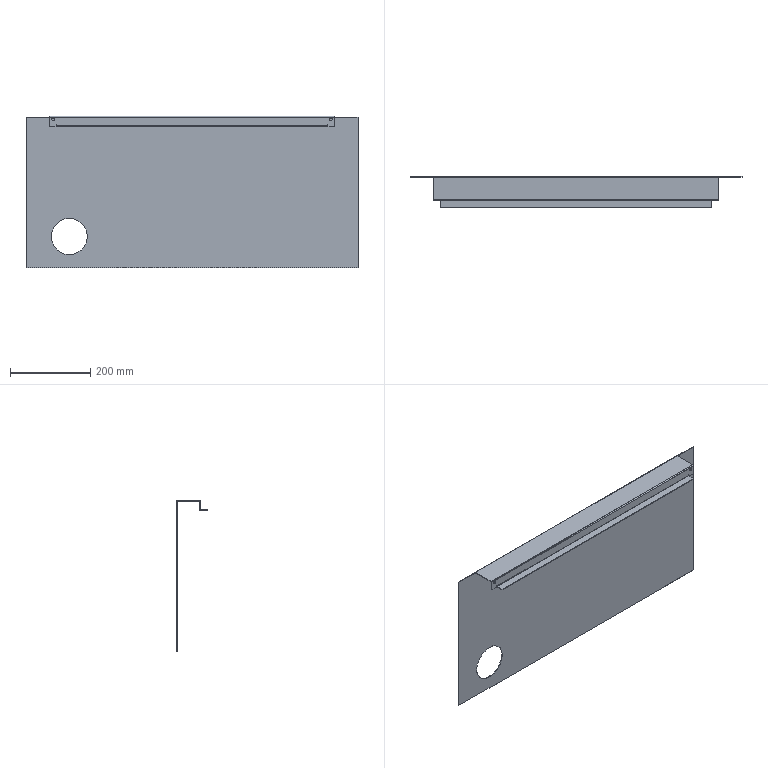Part | STEP file | Electrical Cabinet 3 | 1 solid | 42 faces | box 828 x 78 x 378 mm | volume 749579 mm3 | plane 24 | cylinder 18 | commonest cylinder face diameters 1 x9 7 x4 5 x3 90 x2
STEP:
#1=CARTESIAN_POINT('',(32.62,0.,79.307));
#2=VERTEX_POINT('',#1);
#3=CARTESIAN_POINT('',(32.62,0.,-10.693));
#4=VERTEX_POINT('',#3);
#5=CARTESIAN_POINT('',(32.62,0.,34.307));
#6=DIRECTION('',(0.,-1.,0.));
#7=DIRECTION('',(0.,0.,-1.));
#8=AXIS2_PLACEMENT_3D('',#5,#6,#7);
#9=CIRCLE('',#8,45.);
#10=EDGE_CURVE('',#2,#4,#9,.T.);
#11=ORIENTED_EDGE('',*,*,#10,.F.);
#12=CARTESIAN_POINT('',(32.62,-2.,79.307));
#13=VERTEX_POINT('',#12);
#14=CARTESIAN_POINT('',(32.62,8.,79.307));
#15=DIRECTION('',(0.,-1.,0.));
#16=VECTOR('',#15,1000.);
#17=LINE('',#14,#16);
#18=EDGE_CURVE('',#2,#13,#17,.T.);
#19=ORIENTED_EDGE('',*,*,#18,.T.);
#20=CARTESIAN_POINT('',(32.62,-2.,-10.693));
#21=VERTEX_POINT('',#20);
#22=CARTESIAN_POINT('',(32.62,-2.,34.307));
#23=DIRECTION('',(0.,-1.,0.));
#24=DIRECTION('',(0.,0.,-1.));
#25=AXIS2_PLACEMENT_3D('',#22,#23,#24);
#26=CIRCLE('',#25,45.);
#27=EDGE_CURVE('',#13,#21,#26,.T.);
#28=ORIENTED_EDGE('',*,*,#27,.T.);
#29=CARTESIAN_POINT('',(32.62,8.,-10.693));
#30=DIRECTION('',(0.,-1.,0.));
#31=VECTOR('',#30,1000.);
#32=LINE('',#29,#31);
#33=EDGE_CURVE('',#4,#21,#32,.T.);
#34=ORIENTED_EDGE('',*,*,#33,.F.);
#35=EDGE_LOOP('',(#11,#19,#28,#34));
#36=FACE_OUTER_BOUND('',#35,.T.);
#37=CARTESIAN_POINT('',(32.62,8.,34.307));
#38=DIRECTION('',(0.,-1.,0.));
#39=DIRECTION('',(0.,0.,-1.));
#40=AXIS2_PLACEMENT_3D('',#37,#38,#39);
#41=CYLINDRICAL_SURFACE('',#40,45.);
#42=ADVANCED_FACE('',(#36),#41,.F.);
#43=CARTESIAN_POINT('',(684.62,-58.,322.807));
#44=VERTEX_POINT('',#43);
#45=CARTESIAN_POINT('',(684.62,-58.,329.807));
#46=VERTEX_POINT('',#45);
#47=CARTESIAN_POINT('',(684.62,-58.,326.307));
#48=DIRECTION('',(0.,1.,0.));
#49=DIRECTION('',(0.,0.,-1.));
#50=AXIS2_PLACEMENT_3D('',#47,#48,#49);
#51=CIRCLE('',#50,3.5);
#52=EDGE_CURVE('',#44,#46,#51,.T.);
#53=ORIENTED_EDGE('',*,*,#52,.T.);
#54=CARTESIAN_POINT('',(684.62,-60.,329.807));
#55=VERTEX_POINT('',#54);
#56=CARTESIAN_POINT('',(684.62,-50.,329.807));
#57=DIRECTION('',(0.,-1.,0.));
#58=VECTOR('',#57,1000.);
#59=LINE('',#56,#58);
#60=EDGE_CURVE('',#46,#55,#59,.T.);
#61=ORIENTED_EDGE('',*,*,#60,.T.);
#62=CARTESIAN_POINT('',(684.62,-60.,322.807));
#63=VERTEX_POINT('',#62);
#64=CARTESIAN_POINT('',(684.62,-60.,326.307));
#65=DIRECTION('',(0.,1.,0.));
#66=DIRECTION('',(0.,0.,-1.));
#67=AXIS2_PLACEMENT_3D('',#64,#65,#66);
#68=CIRCLE('',#67,3.5);
#69=EDGE_CURVE('',#63,#55,#68,.T.);
#70=ORIENTED_EDGE('',*,*,#69,.F.);
#71=CARTESIAN_POINT('',(684.62,-50.,322.807));
#72=DIRECTION('',(0.,-1.,0.));
#73=VECTOR('',#72,1000.);
#74=LINE('',#71,#73);
#75=EDGE_CURVE('',#44,#63,#74,.T.);
#76=ORIENTED_EDGE('',*,*,#75,.F.);
#77=EDGE_LOOP('',(#53,#61,#70,#76));
#78=FACE_OUTER_BOUND('',#77,.T.);
#79=CARTESIAN_POINT('',(684.62,-50.,326.307));
#80=DIRECTION('',(0.,-1.,0.));
#81=DIRECTION('',(0.,0.,-1.));
#82=AXIS2_PLACEMENT_3D('',#79,#80,#81);
#83=CYLINDRICAL_SURFACE('',#82,3.5);
#84=ADVANCED_FACE('',(#78),#83,.F.);
#85=CARTESIAN_POINT('',(-7.38,-58.,322.807));
#86=VERTEX_POINT('',#85);
#87=CARTESIAN_POINT('',(-7.38,-58.,329.807));
#88=VERTEX_POINT('',#87);
#89=CARTESIAN_POINT('',(-7.38,-58.,326.307));
#90=DIRECTION('',(0.,1.,0.));
#91=DIRECTION('',(0.,0.,-1.));
#92=AXIS2_PLACEMENT_3D('',#89,#90,#91);
#93=CIRCLE('',#92,3.5);
#94=EDGE_CURVE('',#86,#88,#93,.T.);
#95=ORIENTED_EDGE('',*,*,#94,.T.);
#96=CARTESIAN_POINT('',(-7.38,-60.,329.807));
#97=VERTEX_POINT('',#96);
#98=CARTESIAN_POINT('',(-7.38,-50.,329.807));
#99=DIRECTION('',(0.,-1.,0.));
#100=VECTOR('',#99,1000.);
#101=LINE('',#98,#100);
#102=EDGE_CURVE('',#88,#97,#101,.T.);
#103=ORIENTED_EDGE('',*,*,#102,.T.);
#104=CARTESIAN_POINT('',(-7.38,-60.,322.807));
#105=VERTEX_POINT('',#104);
#106=CARTESIAN_POINT('',(-7.38,-60.,326.307));
#107=DIRECTION('',(0.,1.,0.));
#108=DIRECTION('',(0.,0.,-1.));
#109=AXIS2_PLACEMENT_3D('',#106,#107,#108);
#110=CIRCLE('',#109,3.5);
#111=EDGE_CURVE('',#105,#97,#110,.T.);
#112=ORIENTED_EDGE('',*,*,#111,.F.);
#113=CARTESIAN_POINT('',(-7.38,-50.,322.807));
#114=DIRECTION('',(0.,-1.,0.));
#115=VECTOR('',#114,1000.);
#116=LINE('',#113,#115);
#117=EDGE_CURVE('',#86,#105,#116,.T.);
#118=ORIENTED_EDGE('',*,*,#117,.F.);
#119=EDGE_LOOP('',(#95,#103,#112,#118));
#120=FACE_OUTER_BOUND('',#119,.T.);
#121=CARTESIAN_POINT('',(-7.38,-50.,326.307));
#122=DIRECTION('',(0.,-1.,0.));
#123=DIRECTION('',(0.,0.,-1.));
#124=AXIS2_PLACEMENT_3D('',#121,#122,#123);
#125=CYLINDRICAL_SURFACE('',#124,3.5);
#126=ADVANCED_FACE('',(#120),#125,.F.);
#127=CARTESIAN_POINT('',(677.12,-60.,313.307));
#128=VERTEX_POINT('',#127);
#129=CARTESIAN_POINT('',(677.62,-60.,312.807));
#130=VERTEX_POINT('',#129);
#131=CARTESIAN_POINT('',(677.12,-60.,312.807));
#132=DIRECTION('',(0.,1.,0.));
#133=DIRECTION('',(0.,0.,1.));
#134=AXIS2_PLACEMENT_3D('',#131,#132,#133);
#135=CIRCLE('',#134,0.5);
#136=EDGE_CURVE('',#128,#130,#135,.T.);
#137=ORIENTED_EDGE('',*,*,#136,.F.);
#138=CARTESIAN_POINT('',(677.12,-58.,313.307));
#139=VERTEX_POINT('',#138);
#140=CARTESIAN_POINT('',(677.12,-60.,313.307));
#141=DIRECTION('',(0.,1.,0.));
#142=VECTOR('',#141,1000.);
#143=LINE('',#140,#142);
#144=EDGE_CURVE('',#128,#139,#143,.T.);
#145=ORIENTED_EDGE('',*,*,#144,.T.);
#146=CARTESIAN_POINT('',(677.62,-58.,312.807));
#147=VERTEX_POINT('',#146);
#148=CARTESIAN_POINT('',(677.12,-58.,312.807));
#149=DIRECTION('',(0.,-1.,0.));
#150=DIRECTION('',(0.,0.,1.));
#151=AXIS2_PLACEMENT_3D('',#148,#149,#150);
#152=CIRCLE('',#151,0.5);
#153=EDGE_CURVE('',#147,#139,#152,.T.);
#154=ORIENTED_EDGE('',*,*,#153,.F.);
#155=CARTESIAN_POINT('',(677.62,-60.,312.807));
#156=DIRECTION('',(0.,1.,0.));
#157=VECTOR('',#156,1000.);
#158=LINE('',#155,#157);
#159=EDGE_CURVE('',#130,#147,#158,.T.);
#160=ORIENTED_EDGE('',*,*,#159,.F.);
#161=EDGE_LOOP('',(#137,#145,#154,#160));
#162=FACE_OUTER_BOUND('',#161,.T.);
#163=CARTESIAN_POINT('',(677.12,-60.,312.807));
#164=DIRECTION('',(0.,1.,0.));
#165=DIRECTION('',(0.,0.,1.));
#166=AXIS2_PLACEMENT_3D('',#163,#164,#165);
#167=CYLINDRICAL_SURFACE('',#166,0.5);
#168=ADVANCED_FACE('',(#162),#167,.F.);
#169=CARTESIAN_POINT('',(0.1199,-60.,313.307));
#170=VERTEX_POINT('',#169);
#171=CARTESIAN_POINT('',(0.6199,-60.,312.807));
#172=VERTEX_POINT('',#171);
#173=CARTESIAN_POINT('',(0.1199,-60.,312.807));
#174=DIRECTION('',(0.,1.,0.));
#175=DIRECTION('',(0.,0.,1.));
#176=AXIS2_PLACEMENT_3D('',#173,#174,#175);
#177=CIRCLE('',#176,0.5);
#178=EDGE_CURVE('',#170,#172,#177,.T.);
#179=ORIENTED_EDGE('',*,*,#178,.F.);
#180=CARTESIAN_POINT('',(0.1199,-58.,313.307));
#181=VERTEX_POINT('',#180);
#182=CARTESIAN_POINT('',(0.1199,-60.,313.307));
#183=DIRECTION('',(0.,1.,0.));
#184=VECTOR('',#183,1000.);
#185=LINE('',#182,#184);
#186=EDGE_CURVE('',#170,#181,#185,.T.);
#187=ORIENTED_EDGE('',*,*,#186,.T.);
#188=CARTESIAN_POINT('',(0.6199,-58.,312.807));
#189=VERTEX_POINT('',#188);
#190=CARTESIAN_POINT('',(0.1199,-58.,312.807));
#191=DIRECTION('',(0.,-1.,0.));
#192=DIRECTION('',(0.,0.,1.));
#193=AXIS2_PLACEMENT_3D('',#190,#191,#192);
#194=CIRCLE('',#193,0.5);
#195=EDGE_CURVE('',#189,#181,#194,.T.);
#196=ORIENTED_EDGE('',*,*,#195,.F.);
#197=CARTESIAN_POINT('',(0.6199,-60.,312.807));
#198=DIRECTION('',(0.,1.,0.));
#199=VECTOR('',#198,1000.);
#200=LINE('',#197,#199);
#201=EDGE_CURVE('',#172,#189,#200,.T.);
#202=ORIENTED_EDGE('',*,*,#201,.F.);
#203=EDGE_LOOP('',(#179,#187,#196,#202));
#204=FACE_OUTER_BOUND('',#203,.T.);
#205=CARTESIAN_POINT('',(0.1199,-60.,312.807));
#206=DIRECTION('',(0.,1.,0.));
#207=DIRECTION('',(0.,0.,1.));
#208=AXIS2_PLACEMENT_3D('',#205,#206,#207);
#209=CYLINDRICAL_SURFACE('',#208,0.5);
#210=ADVANCED_FACE('',(#204),#209,.F.);
#211=CARTESIAN_POINT('',(-75.38,-2.,332.307));
#212=VERTEX_POINT('',#211);
#213=CARTESIAN_POINT('',(-18.38,-2.,332.307));
#214=VERTEX_POINT('',#213);
#215=CARTESIAN_POINT('',(0.,-2.,332.307));
#216=DIRECTION('',(1.,0.,0.));
#217=VECTOR('',#216,1000.);
#218=LINE('',#215,#217);
#219=EDGE_CURVE('',#212,#214,#218,.T.);
#220=ORIENTED_EDGE('',*,*,#219,.F.);
#221=CARTESIAN_POINT('',(-75.38,-2.,-43.693));
#222=VERTEX_POINT('',#221);
#223=CARTESIAN_POINT('',(-75.38,-2.,0.));
#224=DIRECTION('',(0.,0.,1.));
#225=VECTOR('',#224,1000.);
#226=LINE('',#223,#225);
#227=EDGE_CURVE('',#222,#212,#226,.T.);
#228=ORIENTED_EDGE('',*,*,#227,.F.);
#229=CARTESIAN_POINT('',(752.62,-2.,-43.693));
#230=VERTEX_POINT('',#229);
#231=CARTESIAN_POINT('',(0.,-2.,-43.693));
#232=DIRECTION('',(-1.,0.,0.));
#233=VECTOR('',#232,1000.);
#234=LINE('',#231,#233);
#235=EDGE_CURVE('',#230,#222,#234,.T.);
#236=ORIENTED_EDGE('',*,*,#235,.F.);
#237=CARTESIAN_POINT('',(752.62,-2.,332.307));
#238=VERTEX_POINT('',#237);
#239=CARTESIAN_POINT('',(752.62,-2.,0.));
#240=DIRECTION('',(0.,0.,-1.));
#241=VECTOR('',#240,1000.);
#242=LINE('',#239,#241);
#243=EDGE_CURVE('',#238,#230,#242,.T.);
#244=ORIENTED_EDGE('',*,*,#243,.F.);
#245=CARTESIAN_POINT('',(695.62,-2.,332.307));
#246=VERTEX_POINT('',#245);
#247=CARTESIAN_POINT('',(0.,-2.,332.307));
#248=DIRECTION('',(1.,0.,0.));
#249=VECTOR('',#248,1000.);
#250=LINE('',#247,#249);
#251=EDGE_CURVE('',#246,#238,#250,.T.);
#252=ORIENTED_EDGE('',*,*,#251,.F.);
#253=CARTESIAN_POINT('',(695.62,-2.,330.807));
#254=VERTEX_POINT('',#253);
#255=CARTESIAN_POINT('',(695.62,-2.,330.807));
#256=DIRECTION('',(0.,0.,1.));
#257=VECTOR('',#256,1000.);
#258=LINE('',#255,#257);
#259=EDGE_CURVE('',#254,#246,#258,.T.);
#260=ORIENTED_EDGE('',*,*,#259,.F.);
#261=CARTESIAN_POINT('',(694.62,-2.,330.807));
#262=VERTEX_POINT('',#261);
#263=CARTESIAN_POINT('',(695.12,-2.,330.807));
#264=DIRECTION('',(0.,1.,0.));
#265=DIRECTION('',(0.,0.,1.));
#266=AXIS2_PLACEMENT_3D('',#263,#264,#265);
#267=CIRCLE('',#266,0.5);
#268=EDGE_CURVE('',#254,#262,#267,.T.);
#269=ORIENTED_EDGE('',*,*,#268,.T.);
#270=CARTESIAN_POINT('',(694.62,-2.,331.807));
#271=VERTEX_POINT('',#270);
#272=CARTESIAN_POINT('',(694.62,-2.,331.807));
#273=DIRECTION('',(0.,0.,-1.));
#274=VECTOR('',#273,1000.);
#275=LINE('',#272,#274);
#276=EDGE_CURVE('',#271,#262,#275,.T.);
#277=ORIENTED_EDGE('',*,*,#276,.F.);
#278=CARTESIAN_POINT('',(-17.38,-2.,331.807));
#279=VERTEX_POINT('',#278);
#280=CARTESIAN_POINT('',(0.,-2.,331.807));
#281=DIRECTION('',(1.,0.,0.));
#282=VECTOR('',#281,1000.);
#283=LINE('',#280,#282);
#284=EDGE_CURVE('',#279,#271,#283,.T.);
#285=ORIENTED_EDGE('',*,*,#284,.F.);
#286=CARTESIAN_POINT('',(-17.38,-2.,330.807));
#287=VERTEX_POINT('',#286);
#288=CARTESIAN_POINT('',(-17.38,-2.,330.807));
#289=DIRECTION('',(0.,0.,1.));
#290=VECTOR('',#289,1000.);
#291=LINE('',#288,#290);
#292=EDGE_CURVE('',#287,#279,#291,.T.);
#293=ORIENTED_EDGE('',*,*,#292,.F.);
#294=CARTESIAN_POINT('',(-18.38,-2.,330.807));
#295=VERTEX_POINT('',#294);
#296=CARTESIAN_POINT('',(-17.88,-2.,330.807));
#297=DIRECTION('',(0.,1.,0.));
#298=DIRECTION('',(0.,0.,1.));
#299=AXIS2_PLACEMENT_3D('',#296,#297,#298);
#300=CIRCLE('',#299,0.5);
#301=EDGE_CURVE('',#287,#295,#300,.T.);
#302=ORIENTED_EDGE('',*,*,#301,.T.);
#303=CARTESIAN_POINT('',(-18.38,-2.,334.307));
#304=DIRECTION('',(0.,0.,-1.));
#305=VECTOR('',#304,1000.);
#306=LINE('',#303,#305);
#307=EDGE_CURVE('',#214,#295,#306,.T.);
#308=ORIENTED_EDGE('',*,*,#307,.F.);
#309=EDGE_LOOP('',(#220,#228,#236,#244,#252,#260,#269,#277,#285,#293,#302,#308));
#310=FACE_OUTER_BOUND('',#309,.T.);
#311=CARTESIAN_POINT('',(32.62,-2.,34.307));
#312=DIRECTION('',(0.,-1.,0.));
#313=DIRECTION('',(0.,0.,-1.));
#314=AXIS2_PLACEMENT_3D('',#311,#312,#313);
#315=CIRCLE('',#314,45.);
#316=EDGE_CURVE('',#21,#13,#315,.T.);
#317=ORIENTED_EDGE('',*,*,#316,.F.);
#318=ORIENTED_EDGE('',*,*,#27,.F.);
#319=EDGE_LOOP('',(#317,#318));
#320=FACE_BOUND('',#319,.T.);
#321=CARTESIAN_POINT('',(0.,-2.,0.));
#322=DIRECTION('',(0.,1.,0.));
#323=DIRECTION('',(0.,0.,1.));
#324=AXIS2_PLACEMENT_3D('',#321,#322,#323);
#325=PLANE('',#324);
#326=ADVANCED_FACE('',(#310,#320),#325,.F.);
#327=CARTESIAN_POINT('',(-75.38,0.,332.307));
#328=VERTEX_POINT('',#327);
#329=CARTESIAN_POINT('',(-18.38,0.,332.307));
#330=VERTEX_POINT('',#329);
#331=CARTESIAN_POINT('',(-18.38,0.,332.307));
#332=DIRECTION('',(1.,0.,0.));
#333=VECTOR('',#332,1000.);
#334=LINE('',#331,#333);
#335=EDGE_CURVE('',#328,#330,#334,.T.);
#336=ORIENTED_EDGE('',*,*,#335,.F.);
#337=CARTESIAN_POINT('',(-75.38,-10.,332.307));
#338=DIRECTION('',(0.,1.,0.));
#339=VECTOR('',#338,1000.);
#340=LINE('',#337,#339);
#341=EDGE_CURVE('',#212,#328,#340,.T.);
#342=ORIENTED_EDGE('',*,*,#341,.F.);
#343=ORIENTED_EDGE('',*,*,#219,.T.);
#344=CARTESIAN_POINT('',(-18.38,-10.,332.307));
#345=DIRECTION('',(0.,-1.,0.));
#346=VECTOR('',#345,1000.);
#347=LINE('',#344,#346);
#348=EDGE_CURVE('',#330,#214,#347,.T.);
#349=ORIENTED_EDGE('',*,*,#348,.F.);
#350=EDGE_LOOP('',(#336,#342,#343,#349));
#351=FACE_OUTER_BOUND('',#350,.T.);
#352=CARTESIAN_POINT('',(-18.38,-10.,332.307));
#353=DIRECTION('',(0.,0.,-1.));
#354=DIRECTION('',(-1.,0.,0.));
#355=AXIS2_PLACEMENT_3D('',#352,#353,#354);
#356=PLANE('',#355);
#357=ADVANCED_FACE('',(#351),#356,.F.);
#358=CARTESIAN_POINT('',(-75.38,0.,-43.693));
#359=VERTEX_POINT('',#358);
#360=CARTESIAN_POINT('',(-75.38,-2.,-43.693));
#361=DIRECTION('',(0.,-1.,0.));
#362=VECTOR('',#361,1000.);
#363=LINE('',#360,#362);
#364=EDGE_CURVE('',#359,#222,#363,.T.);
#365=ORIENTED_EDGE('',*,*,#364,.T.);
#366=ORIENTED_EDGE('',*,*,#227,.T.);
#367=ORIENTED_EDGE('',*,*,#341,.T.);
#368=CARTESIAN_POINT('',(-75.38,0.,-43.693));
#369=DIRECTION('',(0.,0.,-1.));
#370=VECTOR('',#369,1000.);
#371=LINE('',#368,#370);
#372=EDGE_CURVE('',#328,#359,#371,.T.);
#373=ORIENTED_EDGE('',*,*,#372,.T.);
#374=EDGE_LOOP('',(#365,#366,#367,#373));
#375=FACE_OUTER_BOUND('',#374,.T.);
#376=CARTESIAN_POINT('',(-75.38,-2.,-43.693));
#377=DIRECTION('',(-1.,0.,0.));
#378=DIRECTION('',(0.,0.,1.));
#379=AXIS2_PLACEMENT_3D('',#376,#377,#378);
#380=PLANE('',#379);
#381=ADVANCED_FACE('',(#375),#380,.T.);
#382=ORIENTED_EDGE('',*,*,#235,.T.);
#383=ORIENTED_EDGE('',*,*,#364,.F.);
#384=CARTESIAN_POINT('',(752.62,0.,-43.693));
#385=VERTEX_POINT('',#384);
#386=CARTESIAN_POINT('',(-75.38,0.,-43.693));
#387=DIRECTION('',(1.,0.,0.));
#388=VECTOR('',#387,1000.);
#389=LINE('',#386,#388);
#390=EDGE_CURVE('',#359,#385,#389,.T.);
#391=ORIENTED_EDGE('',*,*,#390,.T.);
#392=CARTESIAN_POINT('',(752.62,-2.,-43.693));
#393=DIRECTION('',(0.,-1.,0.));
#394=VECTOR('',#393,1000.);
#395=LINE('',#392,#394);
#396=EDGE_CURVE('',#385,#230,#395,.T.);
#397=ORIENTED_EDGE('',*,*,#396,.T.);
#398=EDGE_LOOP('',(#382,#383,#391,#397));
#399=FACE_OUTER_BOUND('',#398,.T.);
#400=CARTESIAN_POINT('',(-75.38,-2.,-43.693));
#401=DIRECTION('',(0.,0.,-1.));
#402=DIRECTION('',(-1.,0.,0.));
#403=AXIS2_PLACEMENT_3D('',#400,#401,#402);
#404=PLANE('',#403);
#405=ADVANCED_FACE('',(#399),#404,.T.);
#406=ORIENTED_EDGE('',*,*,#396,.F.);
#407=CARTESIAN_POINT('',(752.62,0.,332.307));
#408=VERTEX_POINT('',#407);
#409=CARTESIAN_POINT('',(752.62,0.,-43.693));
#410=DIRECTION('',(0.,0.,1.));
#411=VECTOR('',#410,1000.);
#412=LINE('',#409,#411);
#413=EDGE_CURVE('',#385,#408,#412,.T.);
#414=ORIENTED_EDGE('',*,*,#413,.T.);
#415=CARTESIAN_POINT('',(752.62,-2.,332.307));
#416=DIRECTION('',(0.,-1.,0.));
#417=VECTOR('',#416,1000.);
#418=LINE('',#415,#417);
#419=EDGE_CURVE('',#408,#238,#418,.T.);
#420=ORIENTED_EDGE('',*,*,#419,.T.);
#421=ORIENTED_EDGE('',*,*,#243,.T.);
#422=EDGE_LOOP('',(#406,#414,#420,#421));
#423=FACE_OUTER_BOUND('',#422,.T.);
#424=CARTESIAN_POINT('',(752.62,-2.,-43.693));
#425=DIRECTION('',(1.,0.,0.));
#426=DIRECTION('',(0.,0.,-1.));
#427=AXIS2_PLACEMENT_3D('',#424,#425,#426);
#428=PLANE('',#427);
#429=ADVANCED_FACE('',(#423),#428,.T.);
#430=CARTESIAN_POINT('',(695.62,0.,332.307));
#431=VERTEX_POINT('',#430);
#432=CARTESIAN_POINT('',(695.62,0.,332.307));
#433=DIRECTION('',(1.,0.,0.));
#434=VECTOR('',#433,1000.);
#435=LINE('',#432,#434);
#436=EDGE_CURVE('',#431,#408,#435,.T.);
#437=ORIENTED_EDGE('',*,*,#436,.F.);
#438=CARTESIAN_POINT('',(695.62,-10.,332.307));
#439=DIRECTION('',(0.,1.,0.));
#440=VECTOR('',#439,1000.);
#441=LINE('',#438,#440);
#442=EDGE_CURVE('',#246,#431,#441,.T.);
#443=ORIENTED_EDGE('',*,*,#442,.F.);
#444=ORIENTED_EDGE('',*,*,#251,.T.);
#445=ORIENTED_EDGE('',*,*,#419,.F.);
#446=EDGE_LOOP('',(#437,#443,#444,#445));
#447=FACE_OUTER_BOUND('',#446,.T.);
#448=CARTESIAN_POINT('',(695.62,-10.,332.307));
#449=DIRECTION('',(0.,0.,-1.));
#450=DIRECTION('',(-1.,0.,0.));
#451=AXIS2_PLACEMENT_3D('',#448,#449,#450);
#452=PLANE('',#451);
#453=ADVANCED_FACE('',(#447),#452,.F.);
#454=CARTESIAN_POINT('',(694.62,-2.5,332.307));
#455=VERTEX_POINT('',#454);
#456=CARTESIAN_POINT('',(694.62,-2.5,331.807));
#457=DIRECTION('',(-1.,0.,0.));
#458=DIRECTION('',(0.,0.,1.));
#459=AXIS2_PLACEMENT_3D('',#456,#457,#458);
#460=CIRCLE('',#459,0.5);
#461=EDGE_CURVE('',#455,#271,#460,.T.);
#462=ORIENTED_EDGE('',*,*,#461,.F.);
#463=CARTESIAN_POINT('',(-17.38,-2.5,332.307));
#464=VERTEX_POINT('',#463);
#465=CARTESIAN_POINT('',(-17.38,-2.5,332.307));
#466=DIRECTION('',(1.,0.,0.));
#467=VECTOR('',#466,1000.);
#468=LINE('',#465,#467);
#469=EDGE_CURVE('',#464,#455,#468,.T.);
#470=ORIENTED_EDGE('',*,*,#469,.F.);
#471=CARTESIAN_POINT('',(-17.38,-2.5,331.807));
#472=DIRECTION('',(-1.,0.,0.));
#473=DIRECTION('',(0.,0.,1.));
#474=AXIS2_PLACEMENT_3D('',#471,#472,#473);
#475=CIRCLE('',#474,0.5);
#476=EDGE_CURVE('',#464,#279,#475,.T.);
#477=ORIENTED_EDGE('',*,*,#476,.T.);
#478=ORIENTED_EDGE('',*,*,#284,.T.);
#479=EDGE_LOOP('',(#462,#470,#477,#478));
#480=FACE_OUTER_BOUND('',#479,.T.);
#481=CARTESIAN_POINT('',(-17.38,-2.5,331.807));
#482=DIRECTION('',(-1.,0.,0.));
#483=DIRECTION('',(0.,0.,1.));
#484=AXIS2_PLACEMENT_3D('',#481,#482,#483);
#485=CYLINDRICAL_SURFACE('',#484,0.5);
#486=ADVANCED_FACE('',(#480),#485,.F.);
#487=ORIENTED_EDGE('',*,*,#18,.F.);
#488=CARTESIAN_POINT('',(32.62,0.,34.307));
#489=DIRECTION('',(0.,-1.,0.));
#490=DIRECTION('',(0.,0.,-1.));
#491=AXIS2_PLACEMENT_3D('',#488,#489,#490);
#492=CIRCLE('',#491,45.);
#493=EDGE_CURVE('',#4,#2,#492,.T.);
#494=ORIENTED_EDGE('',*,*,#493,.F.);
#495=ORIENTED_EDGE('',*,*,#33,.T.);
#496=ORIENTED_EDGE('',*,*,#316,.T.);
#497=EDGE_LOOP('',(#487,#494,#495,#496));
#498=FACE_OUTER_BOUND('',#497,.T.);
#499=CARTESIAN_POINT('',(32.62,8.,34.307));
#500=DIRECTION('',(0.,-1.,0.));
#501=DIRECTION('',(0.,0.,-1.));
#502=AXIS2_PLACEMENT_3D('',#499,#500,#501);
#503=CYLINDRICAL_SURFACE('',#502,45.);
#504=ADVANCED_FACE('',(#498),#503,.F.);
#505=CARTESIAN_POINT('',(-18.38,0.,330.807));
#506=VERTEX_POINT('',#505);
#507=CARTESIAN_POINT('',(-18.38,-2.,330.807));
#508=DIRECTION('',(0.,1.,0.));
#509=VECTOR('',#508,1000.);
#510=LINE('',#507,#509);
#511=EDGE_CURVE('',#295,#506,#510,.T.);
#512=ORIENTED_EDGE('',*,*,#511,.T.);
#513=CARTESIAN_POINT('',(-18.38,0.,334.307));
#514=DIRECTION('',(0.,0.,1.));
#515=VECTOR('',#514,1000.);
#516=LINE('',#513,#515);
#517=EDGE_CURVE('',#506,#330,#516,.T.);
#518=ORIENTED_EDGE('',*,*,#517,.T.);
#519=ORIENTED_EDGE('',*,*,#348,.T.);
#520=ORIENTED_EDGE('',*,*,#307,.T.);
#521=EDGE_LOOP('',(#512,#518,#519,#520));
#522=FACE_OUTER_BOUND('',#521,.T.);
#523=CARTESIAN_POINT('',(-18.38,-2.,334.307));
#524=DIRECTION('',(1.,0.,0.));
#525=DIRECTION('',(0.,0.,-1.));
#526=AXIS2_PLACEMENT_3D('',#523,#524,#525);
#527=PLANE('',#526);
#528=ADVANCED_FACE('',(#522),#527,.T.);
#529=ORIENTED_EDGE('',*,*,#390,.F.);
#530=ORIENTED_EDGE('',*,*,#372,.F.);
#531=ORIENTED_EDGE('',*,*,#335,.T.);
#532=ORIENTED_EDGE('',*,*,#517,.F.);
#533=CARTESIAN_POINT('',(-17.38,0.,330.807));
#534=VERTEX_POINT('',#533);
#535=CARTESIAN_POINT('',(-17.88,0.,330.807));
#536=DIRECTION('',(0.,-1.,0.));
#537=DIRECTION('',(0.,0.,1.));
#538=AXIS2_PLACEMENT_3D('',#535,#536,#537);
#539=CIRCLE('',#538,0.5);
#540=EDGE_CURVE('',#506,#534,#539,.T.);
#541=ORIENTED_EDGE('',*,*,#540,.T.);
#542=CARTESIAN_POINT('',(-17.38,0.,331.807));
#543=VERTEX_POINT('',#542);
#544=CARTESIAN_POINT('',(-17.38,0.,330.807));
#545=DIRECTION('',(0.,0.,-1.));
#546=VECTOR('',#545,1000.);
#547=LINE('',#544,#546);
#548=EDGE_CURVE('',#543,#534,#547,.T.);
#549=ORIENTED_EDGE('',*,*,#548,.F.);
#550=CARTESIAN_POINT('',(694.62,0.,331.807));
#551=VERTEX_POINT('',#550);
#552=CARTESIAN_POINT('',(0.,0.,331.807));
#553=DIRECTION('',(1.,0.,0.));
#554=VECTOR('',#553,1000.);
#555=LINE('',#552,#554);
#556=EDGE_CURVE('',#543,#551,#555,.T.);
#557=ORIENTED_EDGE('',*,*,#556,.T.);
#558=CARTESIAN_POINT('',(694.62,0.,330.807));
#559=VERTEX_POINT('',#558);
#560=CARTESIAN_POINT('',(694.62,0.,331.807));
#561=DIRECTION('',(0.,0.,1.));
#562=VECTOR('',#561,1000.);
#563=LINE('',#560,#562);
#564=EDGE_CURVE('',#559,#551,#563,.T.);
#565=ORIENTED_EDGE('',*,*,#564,.F.);
#566=CARTESIAN_POINT('',(695.62,0.,330.807));
#567=VERTEX_POINT('',#566);
#568=CARTESIAN_POINT('',(695.12,0.,330.807));
#569=DIRECTION('',(0.,-1.,0.));
#570=DIRECTION('',(0.,0.,1.));
#571=AXIS2_PLACEMENT_3D('',#568,#569,#570);
#572=CIRCLE('',#571,0.5);
#573=EDGE_CURVE('',#559,#567,#572,.T.);
#574=ORIENTED_EDGE('',*,*,#573,.T.);
#575=CARTESIAN_POINT('',(695.62,0.,0.));
#576=DIRECTION('',(0.,0.,1.));
#577=VECTOR('',#576,1000.);
#578=LINE('',#575,#577);
#579=EDGE_CURVE('',#567,#431,#578,.T.);
#580=ORIENTED_EDGE('',*,*,#579,.T.);
#581=ORIENTED_EDGE('',*,*,#436,.T.);
#582=ORIENTED_EDGE('',*,*,#413,.F.);
#583=EDGE_LOOP('',(#529,#530,#531,#532,#541,#549,#557,#565,#574,#580,#581,#582));
#584=FACE_OUTER_BOUND('',#583,.T.);
#585=ORIENTED_EDGE('',*,*,#493,.T.);
#586=ORIENTED_EDGE('',*,*,#10,.T.);
#587=EDGE_LOOP('',(#585,#586));
#588=FACE_BOUND('',#587,.T.);
#589=CARTESIAN_POINT('',(0.,0.,0.));
#590=DIRECTION('',(0.,1.,0.));
#591=DIRECTION('',(0.,0.,1.));
#592=AXIS2_PLACEMENT_3D('',#589,#590,#591);
#593=PLANE('',#592);
#594=ADVANCED_FACE('',(#584,#588),#593,.T.);
#595=CARTESIAN_POINT('',(695.62,-2.,330.807));
#596=DIRECTION('',(0.,-1.,0.));
#597=VECTOR('',#596,1000.);
#598=LINE('',#595,#597);
#599=EDGE_CURVE('',#567,#254,#598,.T.);
#600=ORIENTED_EDGE('',*,*,#599,.T.);
#601=ORIENTED_EDGE('',*,*,#259,.T.);
#602=ORIENTED_EDGE('',*,*,#442,.T.);
#603=ORIENTED_EDGE('',*,*,#579,.F.);
#604=EDGE_LOOP('',(#600,#601,#602,#603));
#605=FACE_OUTER_BOUND('',#604,.T.);
#606=CARTESIAN_POINT('',(695.62,-2.,330.807));
#607=DIRECTION('',(-1.,0.,0.));
#608=DIRECTION('',(0.,0.,1.));
#609=AXIS2_PLACEMENT_3D('',#606,#607,#608);
#610=PLANE('',#609);
#611=ADVANCED_FACE('',(#605),#610,.T.);
#612=CARTESIAN_POINT('',(-17.38,-57.5,332.307));
#613=VERTEX_POINT('',#612);
#614=CARTESIAN_POINT('',(-17.38,0.,332.307));
#615=DIRECTION('',(0.,-1.,0.));
#616=VECTOR('',#615,1000.);
#617=LINE('',#614,#616);
#618=EDGE_CURVE('',#464,#613,#617,.T.);
#619=ORIENTED_EDGE('',*,*,#618,.F.);
#620=ORIENTED_EDGE('',*,*,#469,.T.);
#621=CARTESIAN_POINT('',(694.62,-57.5,332.307));
#622=VERTEX_POINT('',#621);
#623=CARTESIAN_POINT('',(694.62,0.,332.307));
#624=DIRECTION('',(0.,1.,0.));
#625=VECTOR('',#624,1000.);
#626=LINE('',#623,#625);
#627=EDGE_CURVE('',#622,#455,#626,.T.);
#628=ORIENTED_EDGE('',*,*,#627,.F.);
#629=CARTESIAN_POINT('',(0.,-57.5,332.307));
#630=DIRECTION('',(1.,0.,0.));
#631=VECTOR('',#630,1000.);
#632=LINE('',#629,#631);
#633=EDGE_CURVE('',#613,#622,#632,.T.);
#634=ORIENTED_EDGE('',*,*,#633,.F.);
#635=EDGE_LOOP('',(#619,#620,#628,#634));
#636=FACE_OUTER_BOUND('',#635,.T.);
#637=CARTESIAN_POINT('',(0.,0.,332.307));
#638=DIRECTION('',(0.,0.,1.));
#639=DIRECTION('',(0.,-1.,0.));
#640=AXIS2_PLACEMENT_3D('',#637,#638,#639);
#641=PLANE('',#640);
#642=ADVANCED_FACE('',(#636),#641,.F.);
#643=ORIENTED_EDGE('',*,*,#511,.F.);
#644=ORIENTED_EDGE('',*,*,#301,.F.);
#645=CARTESIAN_POINT('',(-17.38,-2.,330.807));
#646=DIRECTION('',(0.,-1.,0.));
#647=VECTOR('',#646,1000.);
#648=LINE('',#645,#647);
#649=EDGE_CURVE('',#534,#287,#648,.T.);
#650=ORIENTED_EDGE('',*,*,#649,.F.);
#651=ORIENTED_EDGE('',*,*,#540,.F.);
#652=EDGE_LOOP('',(#643,#644,#650,#651));
#653=FACE_OUTER_BOUND('',#652,.T.);
#654=CARTESIAN_POINT('',(-17.88,-2.,330.807));
#655=DIRECTION('',(0.,1.,0.));
#656=DIRECTION('',(0.,0.,1.));
#657=AXIS2_PLACEMENT_3D('',#654,#655,#656);
#658=CYLINDRICAL_SURFACE('',#657,0.5);
#659=ADVANCED_FACE('',(#653),#658,.F.);
#660=CARTESIAN_POINT('',(-17.38,-2.5,334.307));
#661=VERTEX_POINT('',#660);
#662=CARTESIAN_POINT('',(694.62,-2.5,334.307));
#663=VERTEX_POINT('',#662);
#664=CARTESIAN_POINT('',(-17.38,-2.5,334.307));
#665=DIRECTION('',(1.,0.,0.));
#666=VECTOR('',#665,1000.);
#667=LINE('',#664,#666);
#668=EDGE_CURVE('',#661,#663,#667,.T.);
#669=ORIENTED_EDGE('',*,*,#668,.T.);
#670=CARTESIAN_POINT('',(694.62,-2.5,331.807));
#671=DIRECTION('',(-1.,0.,0.));
#672=DIRECTION('',(0.,0.,1.));
#673=AXIS2_PLACEMENT_3D('',#670,#671,#672);
#674=CIRCLE('',#673,2.5);
#675=EDGE_CURVE('',#663,#551,#674,.T.);
#676=ORIENTED_EDGE('',*,*,#675,.T.);
#677=ORIENTED_EDGE('',*,*,#556,.F.);
#678=CARTESIAN_POINT('',(-17.38,-2.5,331.807));
#679=DIRECTION('',(1.,0.,0.));
#680=DIRECTION('',(0.,0.,1.));
#681=AXIS2_PLACEMENT_3D('',#678,#679,#680);
#682=CIRCLE('',#681,2.5);
#683=EDGE_CURVE('',#543,#661,#682,.T.);
#684=ORIENTED_EDGE('',*,*,#683,.T.);
#685=EDGE_LOOP('',(#669,#676,#677,#684));
#686=FACE_OUTER_BOUND('',#685,.T.);
#687=CARTESIAN_POINT('',(-17.38,-2.5,331.807));
#688=DIRECTION('',(-1.,0.,0.));
#689=DIRECTION('',(0.,0.,1.));
#690=AXIS2_PLACEMENT_3D('',#687,#688,#689);
#691=CYLINDRICAL_SURFACE('',#690,2.5);
#692=ADVANCED_FACE('',(#686),#691,.T.);
#693=CARTESIAN_POINT('',(694.62,-2.,330.807));
#694=DIRECTION('',(0.,1.,0.));
#695=VECTOR('',#694,1000.);
#696=LINE('',#693,#695);
#697=EDGE_CURVE('',#262,#559,#696,.T.);
#698=ORIENTED_EDGE('',*,*,#697,.F.);
#699=ORIENTED_EDGE('',*,*,#268,.F.);
#700=ORIENTED_EDGE('',*,*,#599,.F.);
#701=ORIENTED_EDGE('',*,*,#573,.F.);
#702=EDGE_LOOP('',(#698,#699,#700,#701));
#703=FACE_OUTER_BOUND('',#702,.T.);
#704=CARTESIAN_POINT('',(695.12,-2.,330.807));
#705=DIRECTION('',(0.,1.,0.));
#706=DIRECTION('',(0.,0.,1.));
#707=AXIS2_PLACEMENT_3D('',#704,#705,#706);
#708=CYLINDRICAL_SURFACE('',#707,0.5);
#709=ADVANCED_FACE('',(#703),#708,.F.);
#710=CARTESIAN_POINT('',(694.62,-58.,331.807));
#711=VERTEX_POINT('',#710);
#712=CARTESIAN_POINT('',(694.62,-57.5,331.807));
#713=DIRECTION('',(-1.,0.,0.));
#714=DIRECTION('',(0.,0.,1.));
#715=AXIS2_PLACEMENT_3D('',#712,#713,#714);
#716=CIRCLE('',#715,0.5);
#717=EDGE_CURVE('',#711,#622,#716,.T.);
#718=ORIENTED_EDGE('',*,*,#717,.F.);
#719=CARTESIAN_POINT('',(-17.38,-58.,331.807));
#720=VERTEX_POINT('',#719);
#721=CARTESIAN_POINT('',(-17.38,-58.,331.807));
#722=DIRECTION('',(1.,0.,0.));
#723=VECTOR('',#722,1000.);
#724=LINE('',#721,#723);
#725=EDGE_CURVE('',#720,#711,#724,.T.);
#726=ORIENTED_EDGE('',*,*,#725,.F.);
#727=CARTESIAN_POINT('',(-17.38,-57.5,331.807));
#728=DIRECTION('',(-1.,0.,0.));
#729=DIRECTION('',(0.,0.,1.));
#730=AXIS2_PLACEMENT_3D('',#727,#728,#729);
#731=CIRCLE('',#730,0.5);
#732=EDGE_CURVE('',#720,#613,#731,.T.);
#733=ORIENTED_EDGE('',*,*,#732,.T.);
#734=ORIENTED_EDGE('',*,*,#633,.T.);
#735=EDGE_LOOP('',(#718,#726,#733,#734));
#736=FACE_OUTER_BOUND('',#735,.T.);
#737=CARTESIAN_POINT('',(-17.38,-57.5,331.807));
#738=DIRECTION('',(-1.,0.,0.));
#739=DIRECTION('',(0.,0.,1.));
#740=AXIS2_PLACEMENT_3D('',#737,#738,#739);
#741=CYLINDRICAL_SURFACE('',#740,0.5);
#742=ADVANCED_FACE('',(#736),#741,.F.);
#743=CARTESIAN_POINT('',(-17.38,-57.5,334.307));
#744=VERTEX_POINT('',#743);
#745=CARTESIAN_POINT('',(-17.38,-2.,334.307));
#746=DIRECTION('',(0.,1.,0.));
#747=VECTOR('',#746,1000.);
#748=LINE('',#745,#747);
#749=EDGE_CURVE('',#744,#661,#748,.T.);
#750=ORIENTED_EDGE('',*,*,#749,.T.);
#751=ORIENTED_EDGE('',*,*,#683,.F.);
#752=ORIENTED_EDGE('',*,*,#548,.T.);
#753=ORIENTED_EDGE('',*,*,#649,.T.);
#754=ORIENTED_EDGE('',*,*,#292,.T.);
#755=ORIENTED_EDGE('',*,*,#476,.F.);
#756=ORIENTED_EDGE('',*,*,#618,.T.);
#757=ORIENTED_EDGE('',*,*,#732,.F.);
#758=CARTESIAN_POINT('',(-17.38,-58.,309.307));
#759=VERTEX_POINT('',#758);
#760=CARTESIAN_POINT('',(-17.38,-58.,0.));
#761=DIRECTION('',(0.,0.,-1.));
#762=VECTOR('',#761,1000.);
#763=LINE('',#760,#762);
#764=EDGE_CURVE('',#720,#759,#763,.T.);
#765=ORIENTED_EDGE('',*,*,#764,.T.);
#766=CARTESIAN_POINT('',(-17.38,-60.,309.307));
#767=VERTEX_POINT('',#766);
#768=CARTESIAN_POINT('',(-17.38,-60.,309.307));
#769=DIRECTION('',(0.,1.,0.));
#770=VECTOR('',#769,1000.);
#771=LINE('',#768,#770);
#772=EDGE_CURVE('',#767,#759,#771,.T.);
#773=ORIENTED_EDGE('',*,*,#772,.F.);
#774=CARTESIAN_POINT('',(-17.38,-60.,331.807));
#775=VERTEX_POINT('',#774);
#776=CARTESIAN_POINT('',(-17.38,-60.,332.307));
#777=DIRECTION('',(0.,0.,1.));
#778=VECTOR('',#777,1000.);
#779=LINE('',#776,#778);
#780=EDGE_CURVE('',#767,#775,#779,.T.);
#781=ORIENTED_EDGE('',*,*,#780,.T.);
#782=CARTESIAN_POINT('',(-17.38,-57.5,331.807));
#783=DIRECTION('',(1.,0.,0.));
#784=DIRECTION('',(0.,0.,1.));
#785=AXIS2_PLACEMENT_3D('',#782,#783,#784);
#786=CIRCLE('',#785,2.5);
#787=EDGE_CURVE('',#744,#775,#786,.T.);
#788=ORIENTED_EDGE('',*,*,#787,.F.);
#789=EDGE_LOOP('',(#750,#751,#752,#753,#754,#755,#756,#757,#765,#773,#781,#788));
#790=FACE_OUTER_BOUND('',#789,.T.);
#791=CARTESIAN_POINT('',(-17.38,-2.,334.307));
#792=DIRECTION('',(-1.,0.,0.));
#793=DIRECTION('',(0.,-1.,0.));
#794=AXIS2_PLACEMENT_3D('',#791,#792,#793);
#795=PLANE('',#794);
#796=ADVANCED_FACE('',(#790),#795,.T.);
#797=ORIENTED_EDGE('',*,*,#627,.T.);
#798=ORIENTED_EDGE('',*,*,#461,.T.);
#799=ORIENTED_EDGE('',*,*,#276,.T.);
#800=ORIENTED_EDGE('',*,*,#697,.T.);
#801=ORIENTED_EDGE('',*,*,#564,.T.);
#802=ORIENTED_EDGE('',*,*,#675,.F.);
#803=CARTESIAN_POINT('',(694.62,-57.5,334.307));
#804=VERTEX_POINT('',#803);
#805=CARTESIAN_POINT('',(694.62,-60.,334.307));
#806=DIRECTION('',(0.,-1.,0.));
#807=VECTOR('',#806,1000.);
#808=LINE('',#805,#807);
#809=EDGE_CURVE('',#663,#804,#808,.T.);
#810=ORIENTED_EDGE('',*,*,#809,.T.);
#811=CARTESIAN_POINT('',(694.62,-60.,331.807));
#812=VERTEX_POINT('',#811);
#813=CARTESIAN_POINT('',(694.62,-57.5,331.807));
#814=DIRECTION('',(1.,0.,0.));
#815=DIRECTION('',(0.,0.,1.));
#816=AXIS2_PLACEMENT_3D('',#813,#814,#815);
#817=CIRCLE('',#816,2.5);
#818=EDGE_CURVE('',#804,#812,#817,.T.);
#819=ORIENTED_EDGE('',*,*,#818,.T.);
#820=CARTESIAN_POINT('',(694.62,-60.,309.307));
#821=VERTEX_POINT('',#820);
#822=CARTESIAN_POINT('',(694.62,-60.,309.307));
#823=DIRECTION('',(0.,0.,-1.));
#824=VECTOR('',#823,1000.);
#825=LINE('',#822,#824);
#826=EDGE_CURVE('',#812,#821,#825,.T.);
#827=ORIENTED_EDGE('',*,*,#826,.T.);
#828=CARTESIAN_POINT('',(694.62,-58.,309.307));
#829=VERTEX_POINT('',#828);
#830=CARTESIAN_POINT('',(694.62,-60.,309.307));
#831=DIRECTION('',(0.,1.,0.));
#832=VECTOR('',#831,1000.);
#833=LINE('',#830,#832);
#834=EDGE_CURVE('',#821,#829,#833,.T.);
#835=ORIENTED_EDGE('',*,*,#834,.T.);
#836=CARTESIAN_POINT('',(694.62,-58.,0.));
#837=DIRECTION('',(0.,0.,1.));
#838=VECTOR('',#837,1000.);
#839=LINE('',#836,#838);
#840=EDGE_CURVE('',#829,#711,#839,.T.);
#841=ORIENTED_EDGE('',*,*,#840,.T.);
#842=ORIENTED_EDGE('',*,*,#717,.T.);
#843=EDGE_LOOP('',(#797,#798,#799,#800,#801,#802,#810,#819,#827,#835,#841,#842));
#844=FACE_OUTER_BOUND('',#843,.T.);
#845=CARTESIAN_POINT('',(694.62,-60.,334.307));
#846=DIRECTION('',(1.,0.,0.));
#847=DIRECTION('',(0.,0.,-1.));
#848=AXIS2_PLACEMENT_3D('',#845,#846,#847);
#849=PLANE('',#848);
#850=ADVANCED_FACE('',(#844),#849,.T.);
#851=ORIENTED_EDGE('',*,*,#809,.F.);
#852=ORIENTED_EDGE('',*,*,#668,.F.);
#853=ORIENTED_EDGE('',*,*,#749,.F.);
#854=CARTESIAN_POINT('',(0.,-57.5,334.307));
#855=DIRECTION('',(1.,0.,0.));
#856=VECTOR('',#855,1000.);
#857=LINE('',#854,#856);
#858=EDGE_CURVE('',#744,#804,#857,.T.);
#859=ORIENTED_EDGE('',*,*,#858,.T.);
#860=EDGE_LOOP('',(#851,#852,#853,#859));
#861=FACE_OUTER_BOUND('',#860,.T.);
#862=CARTESIAN_POINT('',(0.,0.,334.307));
#863=DIRECTION('',(0.,0.,1.));
#864=DIRECTION('',(0.,-1.,0.));
#865=AXIS2_PLACEMENT_3D('',#862,#863,#864);
#866=PLANE('',#865);
#867=ADVANCED_FACE('',(#861),#866,.T.);
#868=ORIENTED_EDGE('',*,*,#153,.T.);
#869=CARTESIAN_POINT('',(676.62,-58.,312.807));
#870=VERTEX_POINT('',#869);
#871=CARTESIAN_POINT('',(677.12,-58.,312.807));
#872=DIRECTION('',(0.,-1.,0.));
#873=DIRECTION('',(0.,0.,1.));
#874=AXIS2_PLACEMENT_3D('',#871,#872,#873);
#875=CIRCLE('',#874,0.5);
#876=EDGE_CURVE('',#139,#870,#875,.T.);
#877=ORIENTED_EDGE('',*,*,#876,.T.);
#878=CARTESIAN_POINT('',(676.62,-58.,311.807));
#879=VERTEX_POINT('',#878);
#880=CARTESIAN_POINT('',(676.62,-58.,312.807));
#881=DIRECTION('',(0.,0.,1.));
#882=VECTOR('',#881,1000.);
#883=LINE('',#880,#882);
#884=EDGE_CURVE('',#879,#870,#883,.T.);
#885=ORIENTED_EDGE('',*,*,#884,.F.);
#886=CARTESIAN_POINT('',(0.6199,-58.,311.807));
#887=VERTEX_POINT('',#886);
#888=CARTESIAN_POINT('',(0.,-58.,311.807));
#889=DIRECTION('',(1.,0.,0.));
#890=VECTOR('',#889,1000.);
#891=LINE('',#888,#890);
#892=EDGE_CURVE('',#887,#879,#891,.T.);
#893=ORIENTED_EDGE('',*,*,#892,.F.);
#894=CARTESIAN_POINT('',(0.6199,-58.,311.807));
#895=DIRECTION('',(0.,0.,-1.));
#896=VECTOR('',#895,1000.);
#897=LINE('',#894,#896);
#898=EDGE_CURVE('',#189,#887,#897,.T.);
#899=ORIENTED_EDGE('',*,*,#898,.F.);
#900=ORIENTED_EDGE('',*,*,#195,.T.);
#901=CARTESIAN_POINT('',(-0.3801,-58.,312.807));
#902=VERTEX_POINT('',#901);
#903=CARTESIAN_POINT('',(0.1199,-58.,312.807));
#904=DIRECTION('',(0.,-1.,0.));
#905=DIRECTION('',(0.,0.,1.));
#906=AXIS2_PLACEMENT_3D('',#903,#904,#905);
#907=CIRCLE('',#906,0.5);
#908=EDGE_CURVE('',#181,#902,#907,.T.);
#909=ORIENTED_EDGE('',*,*,#908,.T.);
#910=CARTESIAN_POINT('',(-0.3801,-58.,309.307));
#911=VERTEX_POINT('',#910);
#912=CARTESIAN_POINT('',(-0.3801,-58.,0.));
#913=DIRECTION('',(0.,0.,1.));
#914=VECTOR('',#913,1000.);
#915=LINE('',#912,#914);
#916=EDGE_CURVE('',#911,#902,#915,.T.);
#917=ORIENTED_EDGE('',*,*,#916,.F.);
#918=CARTESIAN_POINT('',(0.,-58.,309.307));
#919=DIRECTION('',(1.,0.,0.));
#920=VECTOR('',#919,1000.);
#921=LINE('',#918,#920);
#922=EDGE_CURVE('',#759,#911,#921,.T.);
#923=ORIENTED_EDGE('',*,*,#922,.F.);
#924=ORIENTED_EDGE('',*,*,#764,.F.);
#925=ORIENTED_EDGE('',*,*,#725,.T.);
#926=ORIENTED_EDGE('',*,*,#840,.F.);
#927=CARTESIAN_POINT('',(677.62,-58.,309.307));
#928=VERTEX_POINT('',#927);
#929=CARTESIAN_POINT('',(0.,-58.,309.307));
#930=DIRECTION('',(1.,0.,0.));
#931=VECTOR('',#930,1000.);
#932=LINE('',#929,#931);
#933=EDGE_CURVE('',#928,#829,#932,.T.);
#934=ORIENTED_EDGE('',*,*,#933,.F.);
#935=CARTESIAN_POINT('',(677.62,-58.,0.));
#936=DIRECTION('',(0.,0.,-1.));
#937=VECTOR('',#936,1000.);
#938=LINE('',#935,#937);
#939=EDGE_CURVE('',#147,#928,#938,.T.);
#940=ORIENTED_EDGE('',*,*,#939,.F.);
#941=EDGE_LOOP('',(#868,#877,#885,#893,#899,#900,#909,#917,#923,#924,#925,#926,#934,#940));
#942=FACE_OUTER_BOUND('',#941,.T.);
#943=ORIENTED_EDGE('',*,*,#52,.F.);
#944=CARTESIAN_POINT('',(684.62,-58.,326.307));
#945=DIRECTION('',(0.,1.,0.));
#946=DIRECTION('',(0.,0.,-1.));
#947=AXIS2_PLACEMENT_3D('',#944,#945,#946);
#948=CIRCLE('',#947,3.5);
#949=EDGE_CURVE('',#46,#44,#948,.T.);
#950=ORIENTED_EDGE('',*,*,#949,.F.);
#951=EDGE_LOOP('',(#943,#950));
#952=FACE_BOUND('',#951,.T.);
#953=ORIENTED_EDGE('',*,*,#94,.F.);
#954=CARTESIAN_POINT('',(-7.38,-58.,326.307));
#955=DIRECTION('',(0.,1.,0.));
#956=DIRECTION('',(0.,0.,-1.));
#957=AXIS2_PLACEMENT_3D('',#954,#955,#956);
#958=CIRCLE('',#957,3.5);
#959=EDGE_CURVE('',#88,#86,#958,.T.);
#960=ORIENTED_EDGE('',*,*,#959,.F.);
#961=EDGE_LOOP('',(#953,#960));
#962=FACE_BOUND('',#961,.T.);
#963=CARTESIAN_POINT('',(0.,-58.,0.));
#964=DIRECTION('',(0.,-1.,0.));
#965=DIRECTION('',(0.,0.,-1.));
#966=AXIS2_PLACEMENT_3D('',#963,#964,#965);
#967=PLANE('',#966);
#968=ADVANCED_FACE('',(#942,#952,#962),#967,.F.);
#969=CARTESIAN_POINT('',(-17.38,-60.,331.807));
#970=DIRECTION('',(1.,0.,0.));
#971=VECTOR('',#970,1000.);
#972=LINE('',#969,#971);
#973=EDGE_CURVE('',#775,#812,#972,.T.);
#974=ORIENTED_EDGE('',*,*,#973,.T.);
#975=ORIENTED_EDGE('',*,*,#818,.F.);
#976=ORIENTED_EDGE('',*,*,#858,.F.);
#977=ORIENTED_EDGE('',*,*,#787,.T.);
#978=EDGE_LOOP('',(#974,#975,#976,#977));
#979=FACE_OUTER_BOUND('',#978,.T.);
#980=CARTESIAN_POINT('',(-17.38,-57.5,331.807));
#981=DIRECTION('',(-1.,0.,0.));
#982=DIRECTION('',(0.,0.,1.));
#983=AXIS2_PLACEMENT_3D('',#980,#981,#982);
#984=CYLINDRICAL_SURFACE('',#983,2.5);
#985=ADVANCED_FACE('',(#979),#984,.T.);
#986=CARTESIAN_POINT('',(677.62,-60.,309.307));
#987=VERTEX_POINT('',#986);
#988=CARTESIAN_POINT('',(677.62,-60.,309.307));
#989=DIRECTION('',(0.,-1.,0.));
#990=VECTOR('',#989,1000.);
#991=LINE('',#988,#990);
#992=EDGE_CURVE('',#928,#987,#991,.T.);
#993=ORIENTED_EDGE('',*,*,#992,.T.);
#994=CARTESIAN_POINT('',(677.62,-60.,309.307));
#995=DIRECTION('',(0.,0.,1.));
#996=VECTOR('',#995,1000.);
#997=LINE('',#994,#996);
#998=EDGE_CURVE('',#987,#130,#997,.T.);
#999=ORIENTED_EDGE('',*,*,#998,.T.);
#1000=ORIENTED_EDGE('',*,*,#159,.T.);
#1001=ORIENTED_EDGE('',*,*,#939,.T.);
#1002=EDGE_LOOP('',(#993,#999,#1000,#1001));
#1003=FACE_OUTER_BOUND('',#1002,.T.);
#1004=CARTESIAN_POINT('',(677.62,-60.,309.307));
#1005=DIRECTION('',(-1.,0.,0.));
#1006=DIRECTION('',(0.,0.,1.));
#1007=AXIS2_PLACEMENT_3D('',#1004,#1005,#1006);
#1008=PLANE('',#1007);
#1009=ADVANCED_FACE('',(#1003),#1008,.T.);
#1010=CARTESIAN_POINT('',(676.62,-60.5,309.307));
#1011=VERTEX_POINT('',#1010);
#1012=CARTESIAN_POINT('',(0.6199,-60.5,309.307));
#1013=VERTEX_POINT('',#1012);
#1014=CARTESIAN_POINT('',(676.62,-60.5,309.307));
#1015=DIRECTION('',(-1.,0.,0.));
#1016=VECTOR('',#1015,1000.);
#1017=LINE('',#1014,#1016);
#1018=EDGE_CURVE('',#1011,#1013,#1017,.T.);
#1019=ORIENTED_EDGE('',*,*,#1018,.T.);
#1020=CARTESIAN_POINT('',(0.6199,-60.5,311.807));
#1021=DIRECTION('',(1.,0.,0.));
#1022=DIRECTION('',(0.,1.,0.));
#1023=AXIS2_PLACEMENT_3D('',#1020,#1021,#1022);
#1024=CIRCLE('',#1023,2.5);
#1025=EDGE_CURVE('',#1013,#887,#1024,.T.);
#1026=ORIENTED_EDGE('',*,*,#1025,.T.);
#1027=ORIENTED_EDGE('',*,*,#892,.T.);
#1028=CARTESIAN_POINT('',(676.62,-60.5,311.807));
#1029=DIRECTION('',(-1.,0.,0.));
#1030=DIRECTION('',(0.,1.,0.));
#1031=AXIS2_PLACEMENT_3D('',#1028,#1029,#1030);
#1032=CIRCLE('',#1031,2.5);
#1033=EDGE_CURVE('',#879,#1011,#1032,.T.);
#1034=ORIENTED_EDGE('',*,*,#1033,.T.);
#1035=EDGE_LOOP('',(#1019,#1026,#1027,#1034));
#1036=FACE_OUTER_BOUND('',#1035,.T.);
#1037=CARTESIAN_POINT('',(676.62,-60.5,311.807));
#1038=DIRECTION('',(1.,0.,0.));
#1039=DIRECTION('',(0.,1.,0.));
#1040=AXIS2_PLACEMENT_3D('',#1037,#1038,#1039);
#1041=CYLINDRICAL_SURFACE('',#1040,2.5);
#1042=ADVANCED_FACE('',(#1036),#1041,.T.);
#1043=CARTESIAN_POINT('',(-0.3801,-60.,312.807));
#1044=VERTEX_POINT('',#1043);
#1045=CARTESIAN_POINT('',(-0.3801,-60.,312.807));
#1046=DIRECTION('',(0.,-1.,0.));
#1047=VECTOR('',#1046,1000.);
#1048=LINE('',#1045,#1047);
#1049=EDGE_CURVE('',#902,#1044,#1048,.T.);
#1050=ORIENTED_EDGE('',*,*,#1049,.T.);
#1051=CARTESIAN_POINT('',(-0.3801,-60.,309.307));
#1052=VERTEX_POINT('',#1051);
#1053=CARTESIAN_POINT('',(-0.3801,-60.,312.807));
#1054=DIRECTION('',(0.,0.,-1.));
#1055=VECTOR('',#1054,1000.);
#1056=LINE('',#1053,#1055);
#1057=EDGE_CURVE('',#1044,#1052,#1056,.T.);
#1058=ORIENTED_EDGE('',*,*,#1057,.T.);
#1059=CARTESIAN_POINT('',(-0.3801,-60.,309.307));
#1060=DIRECTION('',(0.,1.,0.));
#1061=VECTOR('',#1060,1000.);
#1062=LINE('',#1059,#1061);
#1063=EDGE_CURVE('',#1052,#911,#1062,.T.);
#1064=ORIENTED_EDGE('',*,*,#1063,.T.);
#1065=ORIENTED_EDGE('',*,*,#916,.T.);
#1066=EDGE_LOOP('',(#1050,#1058,#1064,#1065));
#1067=FACE_OUTER_BOUND('',#1066,.T.);
#1068=CARTESIAN_POINT('',(-0.3801,-60.,312.807));
#1069=DIRECTION('',(1.,0.,0.));
#1070=DIRECTION('',(0.,0.,-1.));
#1071=AXIS2_PLACEMENT_3D('',#1068,#1069,#1070);
#1072=PLANE('',#1071);
#1073=ADVANCED_FACE('',(#1067),#1072,.T.);
#1074=CARTESIAN_POINT('',(-17.38,-60.,309.307));
#1075=DIRECTION('',(-1.,0.,0.));
#1076=VECTOR('',#1075,1000.);
#1077=LINE('',#1074,#1076);
#1078=EDGE_CURVE('',#1052,#767,#1077,.T.);
#1079=ORIENTED_EDGE('',*,*,#1078,.T.);
#1080=ORIENTED_EDGE('',*,*,#772,.T.);
#1081=ORIENTED_EDGE('',*,*,#922,.T.);
#1082=ORIENTED_EDGE('',*,*,#1063,.F.);
#1083=EDGE_LOOP('',(#1079,#1080,#1081,#1082));
#1084=FACE_OUTER_BOUND('',#1083,.T.);
#1085=CARTESIAN_POINT('',(-17.38,-60.,309.307));
#1086=DIRECTION('',(0.,0.,-1.));
#1087=DIRECTION('',(0.,1.,0.));
#1088=AXIS2_PLACEMENT_3D('',#1085,#1086,#1087);
#1089=PLANE('',#1088);
#1090=ADVANCED_FACE('',(#1084),#1089,.T.);
#1091=ORIENTED_EDGE('',*,*,#933,.T.);
#1092=ORIENTED_EDGE('',*,*,#834,.F.);
#1093=CARTESIAN_POINT('',(-17.38,-60.,309.307));
#1094=DIRECTION('',(-1.,0.,0.));
#1095=VECTOR('',#1094,1000.);
#1096=LINE('',#1093,#1095);
#1097=EDGE_CURVE('',#821,#987,#1096,.T.);
#1098=ORIENTED_EDGE('',*,*,#1097,.T.);
#1099=ORIENTED_EDGE('',*,*,#992,.F.);
#1100=EDGE_LOOP('',(#1091,#1092,#1098,#1099));
#1101=FACE_OUTER_BOUND('',#1100,.T.);
#1102=CARTESIAN_POINT('',(-17.38,-60.,309.307));
#1103=DIRECTION('',(0.,0.,-1.));
#1104=DIRECTION('',(0.,1.,0.));
#1105=AXIS2_PLACEMENT_3D('',#1102,#1103,#1104);
#1106=PLANE('',#1105);
#1107=ADVANCED_FACE('',(#1101),#1106,.T.);
#1108=ORIENTED_EDGE('',*,*,#60,.F.);
#1109=ORIENTED_EDGE('',*,*,#949,.T.);
#1110=ORIENTED_EDGE('',*,*,#75,.T.);
#1111=CARTESIAN_POINT('',(684.62,-60.,326.307));
#1112=DIRECTION('',(0.,1.,0.));
#1113=DIRECTION('',(0.,0.,-1.));
#1114=AXIS2_PLACEMENT_3D('',#1111,#1112,#1113);
#1115=CIRCLE('',#1114,3.5);
#1116=EDGE_CURVE('',#55,#63,#1115,.T.);
#1117=ORIENTED_EDGE('',*,*,#1116,.F.);
#1118=EDGE_LOOP('',(#1108,#1109,#1110,#1117));
#1119=FACE_OUTER_BOUND('',#1118,.T.);
#1120=CARTESIAN_POINT('',(684.62,-50.,326.307));
#1121=DIRECTION('',(0.,-1.,0.));
#1122=DIRECTION('',(0.,0.,-1.));
#1123=AXIS2_PLACEMENT_3D('',#1120,#1121,#1122);
#1124=CYLINDRICAL_SURFACE('',#1123,3.5);
#1125=ADVANCED_FACE('',(#1119),#1124,.F.);
#1126=ORIENTED_EDGE('',*,*,#102,.F.);
#1127=ORIENTED_EDGE('',*,*,#959,.T.);
#1128=ORIENTED_EDGE('',*,*,#117,.T.);
#1129=CARTESIAN_POINT('',(-7.38,-60.,326.307));
#1130=DIRECTION('',(0.,1.,0.));
#1131=DIRECTION('',(0.,0.,-1.));
#1132=AXIS2_PLACEMENT_3D('',#1129,#1130,#1131);
#1133=CIRCLE('',#1132,3.5);
#1134=EDGE_CURVE('',#97,#105,#1133,.T.);
#1135=ORIENTED_EDGE('',*,*,#1134,.F.);
#1136=EDGE_LOOP('',(#1126,#1127,#1128,#1135));
#1137=FACE_OUTER_BOUND('',#1136,.T.);
#1138=CARTESIAN_POINT('',(-7.38,-50.,326.307));
#1139=DIRECTION('',(0.,-1.,0.));
#1140=DIRECTION('',(0.,0.,-1.));
#1141=AXIS2_PLACEMENT_3D('',#1138,#1139,#1140);
#1142=CYLINDRICAL_SURFACE('',#1141,3.5);
#1143=ADVANCED_FACE('',(#1137),#1142,.F.);
#1144=CARTESIAN_POINT('',(676.62,-60.,312.807));
#1145=VERTEX_POINT('',#1144);
#1146=CARTESIAN_POINT('',(676.62,-60.,311.807));
#1147=VERTEX_POINT('',#1146);
#1148=CARTESIAN_POINT('',(676.62,-60.,312.807));
#1149=DIRECTION('',(0.,0.,-1.));
#1150=VECTOR('',#1149,1000.);
#1151=LINE('',#1148,#1150);
#1152=EDGE_CURVE('',#1145,#1147,#1151,.T.);
#1153=ORIENTED_EDGE('',*,*,#1152,.F.);
#1154=CARTESIAN_POINT('',(677.12,-60.,312.807));
#1155=DIRECTION('',(0.,1.,0.));
#1156=DIRECTION('',(0.,0.,1.));
#1157=AXIS2_PLACEMENT_3D('',#1154,#1155,#1156);
#1158=CIRCLE('',#1157,0.5);
#1159=EDGE_CURVE('',#1145,#128,#1158,.T.);
#1160=ORIENTED_EDGE('',*,*,#1159,.T.);
#1161=ORIENTED_EDGE('',*,*,#136,.T.);
#1162=ORIENTED_EDGE('',*,*,#998,.F.);
#1163=ORIENTED_EDGE('',*,*,#1097,.F.);
#1164=ORIENTED_EDGE('',*,*,#826,.F.);
#1165=ORIENTED_EDGE('',*,*,#973,.F.);
#1166=ORIENTED_EDGE('',*,*,#780,.F.);
#1167=ORIENTED_EDGE('',*,*,#1078,.F.);
#1168=ORIENTED_EDGE('',*,*,#1057,.F.);
#1169=CARTESIAN_POINT('',(0.1199,-60.,312.807));
#1170=DIRECTION('',(0.,1.,0.));
#1171=DIRECTION('',(0.,0.,1.));
#1172=AXIS2_PLACEMENT_3D('',#1169,#1170,#1171);
#1173=CIRCLE('',#1172,0.5);
#1174=EDGE_CURVE('',#1044,#170,#1173,.T.);
#1175=ORIENTED_EDGE('',*,*,#1174,.T.);
#1176=ORIENTED_EDGE('',*,*,#178,.T.);
#1177=CARTESIAN_POINT('',(0.6199,-60.,311.807));
#1178=VERTEX_POINT('',#1177);
#1179=CARTESIAN_POINT('',(0.6199,-60.,311.807));
#1180=DIRECTION('',(0.,0.,1.));
#1181=VECTOR('',#1180,1000.);
#1182=LINE('',#1179,#1181);
#1183=EDGE_CURVE('',#1178,#172,#1182,.T.);
#1184=ORIENTED_EDGE('',*,*,#1183,.F.);
#1185=CARTESIAN_POINT('',(0.,-60.,311.807));
#1186=DIRECTION('',(1.,0.,0.));
#1187=VECTOR('',#1186,1000.);
#1188=LINE('',#1185,#1187);
#1189=EDGE_CURVE('',#1178,#1147,#1188,.T.);
#1190=ORIENTED_EDGE('',*,*,#1189,.T.);
#1191=EDGE_LOOP('',(#1153,#1160,#1161,#1162,#1163,#1164,#1165,#1166,#1167,#1168,#1175,#1176,#1184,#1190));
#1192=FACE_OUTER_BOUND('',#1191,.T.);
#1193=ORIENTED_EDGE('',*,*,#69,.T.);
#1194=ORIENTED_EDGE('',*,*,#1116,.T.);
#1195=EDGE_LOOP('',(#1193,#1194));
#1196=FACE_BOUND('',#1195,.T.);
#1197=ORIENTED_EDGE('',*,*,#111,.T.);
#1198=ORIENTED_EDGE('',*,*,#1134,.T.);
#1199=EDGE_LOOP('',(#1197,#1198));
#1200=FACE_BOUND('',#1199,.T.);
#1201=CARTESIAN_POINT('',(0.,-60.,0.));
#1202=DIRECTION('',(0.,-1.,0.));
#1203=DIRECTION('',(0.,0.,-1.));
#1204=AXIS2_PLACEMENT_3D('',#1201,#1202,#1203);
#1205=PLANE('',#1204);
#1206=ADVANCED_FACE('',(#1192,#1196,#1200),#1205,.T.);
#1207=ORIENTED_EDGE('',*,*,#144,.F.);
#1208=ORIENTED_EDGE('',*,*,#1159,.F.);
#1209=CARTESIAN_POINT('',(676.62,-60.,312.807));
#1210=DIRECTION('',(0.,-1.,0.));
#1211=VECTOR('',#1210,1000.);
#1212=LINE('',#1209,#1211);
#1213=EDGE_CURVE('',#870,#1145,#1212,.T.);
#1214=ORIENTED_EDGE('',*,*,#1213,.F.);
#1215=ORIENTED_EDGE('',*,*,#876,.F.);
#1216=EDGE_LOOP('',(#1207,#1208,#1214,#1215));
#1217=FACE_OUTER_BOUND('',#1216,.T.);
#1218=CARTESIAN_POINT('',(677.12,-60.,312.807));
#1219=DIRECTION('',(0.,1.,0.));
#1220=DIRECTION('',(0.,0.,1.));
#1221=AXIS2_PLACEMENT_3D('',#1218,#1219,#1220);
#1222=CYLINDRICAL_SURFACE('',#1221,0.5);
#1223=ADVANCED_FACE('',(#1217),#1222,.F.);
#1224=CARTESIAN_POINT('',(0.6199,-60.5,311.307));
#1225=VERTEX_POINT('',#1224);
#1226=CARTESIAN_POINT('',(0.6199,-60.5,311.807));
#1227=DIRECTION('',(1.,0.,0.));
#1228=DIRECTION('',(0.,1.,0.));
#1229=AXIS2_PLACEMENT_3D('',#1226,#1227,#1228);
#1230=CIRCLE('',#1229,0.5);
#1231=EDGE_CURVE('',#1225,#1178,#1230,.T.);
#1232=ORIENTED_EDGE('',*,*,#1231,.T.);
#1233=ORIENTED_EDGE('',*,*,#1183,.T.);
#1234=ORIENTED_EDGE('',*,*,#201,.T.);
#1235=ORIENTED_EDGE('',*,*,#898,.T.);
#1236=ORIENTED_EDGE('',*,*,#1025,.F.);
#1237=CARTESIAN_POINT('',(0.6199,-78.,309.307));
#1238=VERTEX_POINT('',#1237);
#1239=CARTESIAN_POINT('',(0.6199,0.,309.307));
#1240=DIRECTION('',(0.,1.,0.));
#1241=VECTOR('',#1240,1000.);
#1242=LINE('',#1239,#1241);
#1243=EDGE_CURVE('',#1238,#1013,#1242,.T.);
#1244=ORIENTED_EDGE('',*,*,#1243,.F.);
#1245=CARTESIAN_POINT('',(0.6199,-78.,311.307));
#1246=VERTEX_POINT('',#1245);
#1247=CARTESIAN_POINT('',(0.6199,-78.,309.307));
#1248=DIRECTION('',(0.,0.,1.));
#1249=VECTOR('',#1248,1000.);
#1250=LINE('',#1247,#1249);
#1251=EDGE_CURVE('',#1238,#1246,#1250,.T.);
#1252=ORIENTED_EDGE('',*,*,#1251,.T.);
#1253=CARTESIAN_POINT('',(0.6199,-78.,311.307));
#1254=DIRECTION('',(0.,1.,0.));
#1255=VECTOR('',#1254,1000.);
#1256=LINE('',#1253,#1255);
#1257=EDGE_CURVE('',#1246,#1225,#1256,.T.);
#1258=ORIENTED_EDGE('',*,*,#1257,.T.);
#1259=EDGE_LOOP('',(#1232,#1233,#1234,#1235,#1236,#1244,#1252,#1258));
#1260=FACE_OUTER_BOUND('',#1259,.T.);
#1261=CARTESIAN_POINT('',(0.6199,-60.5,311.807));
#1262=DIRECTION('',(-1.,0.,0.));
#1263=DIRECTION('',(0.,-1.,0.));
#1264=AXIS2_PLACEMENT_3D('',#1261,#1262,#1263);
#1265=PLANE('',#1264);
#1266=ADVANCED_FACE('',(#1260),#1265,.T.);
#1267=CARTESIAN_POINT('',(676.62,-78.,309.307));
#1268=VERTEX_POINT('',#1267);
#1269=CARTESIAN_POINT('',(676.62,0.,309.307));
#1270=DIRECTION('',(0.,-1.,0.));
#1271=VECTOR('',#1270,1000.);
#1272=LINE('',#1269,#1271);
#1273=EDGE_CURVE('',#1011,#1268,#1272,.T.);
#1274=ORIENTED_EDGE('',*,*,#1273,.T.);
#1275=CARTESIAN_POINT('',(0.,-78.,309.307));
#1276=DIRECTION('',(-1.,0.,0.));
#1277=VECTOR('',#1276,1000.);
#1278=LINE('',#1275,#1277);
#1279=EDGE_CURVE('',#1268,#1238,#1278,.T.);
#1280=ORIENTED_EDGE('',*,*,#1279,.T.);
#1281=ORIENTED_EDGE('',*,*,#1243,.T.);
#1282=ORIENTED_EDGE('',*,*,#1018,.F.);
#1283=EDGE_LOOP('',(#1274,#1280,#1281,#1282));
#1284=FACE_OUTER_BOUND('',#1283,.T.);
#1285=CARTESIAN_POINT('',(0.,0.,309.307));
#1286=DIRECTION('',(0.,0.,-1.));
#1287=DIRECTION('',(0.,1.,0.));
#1288=AXIS2_PLACEMENT_3D('',#1285,#1286,#1287);
#1289=PLANE('',#1288);
#1290=ADVANCED_FACE('',(#1284),#1289,.T.);
#1291=CARTESIAN_POINT('',(676.62,-60.5,311.307));
#1292=VERTEX_POINT('',#1291);
#1293=CARTESIAN_POINT('',(676.62,-60.5,311.807));
#1294=DIRECTION('',(1.,0.,0.));
#1295=DIRECTION('',(0.,1.,0.));
#1296=AXIS2_PLACEMENT_3D('',#1293,#1294,#1295);
#1297=CIRCLE('',#1296,0.5);
#1298=EDGE_CURVE('',#1292,#1147,#1297,.T.);
#1299=ORIENTED_EDGE('',*,*,#1298,.F.);
#1300=CARTESIAN_POINT('',(676.62,-78.,311.307));
#1301=VERTEX_POINT('',#1300);
#1302=CARTESIAN_POINT('',(676.62,-60.,311.307));
#1303=DIRECTION('',(0.,-1.,0.));
#1304=VECTOR('',#1303,1000.);
#1305=LINE('',#1302,#1304);
#1306=EDGE_CURVE('',#1292,#1301,#1305,.T.);
#1307=ORIENTED_EDGE('',*,*,#1306,.T.);
#1308=CARTESIAN_POINT('',(676.62,-78.,309.307));
#1309=DIRECTION('',(0.,0.,1.));
#1310=VECTOR('',#1309,1000.);
#1311=LINE('',#1308,#1310);
#1312=EDGE_CURVE('',#1268,#1301,#1311,.T.);
#1313=ORIENTED_EDGE('',*,*,#1312,.F.);
#1314=ORIENTED_EDGE('',*,*,#1273,.F.);
#1315=ORIENTED_EDGE('',*,*,#1033,.F.);
#1316=ORIENTED_EDGE('',*,*,#884,.T.);
#1317=ORIENTED_EDGE('',*,*,#1213,.T.);
#1318=ORIENTED_EDGE('',*,*,#1152,.T.);
#1319=EDGE_LOOP('',(#1299,#1307,#1313,#1314,#1315,#1316,#1317,#1318));
#1320=FACE_OUTER_BOUND('',#1319,.T.);
#1321=CARTESIAN_POINT('',(676.62,-60.5,311.807));
#1322=DIRECTION('',(-1.,0.,0.));
#1323=DIRECTION('',(0.,-1.,0.));
#1324=AXIS2_PLACEMENT_3D('',#1321,#1322,#1323);
#1325=PLANE('',#1324);
#1326=ADVANCED_FACE('',(#1320),#1325,.F.);
#1327=ORIENTED_EDGE('',*,*,#186,.F.);
#1328=ORIENTED_EDGE('',*,*,#1174,.F.);
#1329=ORIENTED_EDGE('',*,*,#1049,.F.);
#1330=ORIENTED_EDGE('',*,*,#908,.F.);
#1331=EDGE_LOOP('',(#1327,#1328,#1329,#1330));
#1332=FACE_OUTER_BOUND('',#1331,.T.);
#1333=CARTESIAN_POINT('',(0.1199,-60.,312.807));
#1334=DIRECTION('',(0.,1.,0.));
#1335=DIRECTION('',(0.,0.,1.));
#1336=AXIS2_PLACEMENT_3D('',#1333,#1334,#1335);
#1337=CYLINDRICAL_SURFACE('',#1336,0.5);
#1338=ADVANCED_FACE('',(#1332),#1337,.F.);
#1339=ORIENTED_EDGE('',*,*,#1231,.F.);
#1340=CARTESIAN_POINT('',(676.62,-60.5,311.307));
#1341=DIRECTION('',(-1.,0.,0.));
#1342=VECTOR('',#1341,1000.);
#1343=LINE('',#1340,#1342);
#1344=EDGE_CURVE('',#1292,#1225,#1343,.T.);
#1345=ORIENTED_EDGE('',*,*,#1344,.F.);
#1346=ORIENTED_EDGE('',*,*,#1298,.T.);
#1347=ORIENTED_EDGE('',*,*,#1189,.F.);
#1348=EDGE_LOOP('',(#1339,#1345,#1346,#1347));
#1349=FACE_OUTER_BOUND('',#1348,.T.);
#1350=CARTESIAN_POINT('',(676.62,-60.5,311.807));
#1351=DIRECTION('',(1.,0.,0.));
#1352=DIRECTION('',(0.,1.,0.));
#1353=AXIS2_PLACEMENT_3D('',#1350,#1351,#1352);
#1354=CYLINDRICAL_SURFACE('',#1353,0.5);
#1355=ADVANCED_FACE('',(#1349),#1354,.F.);
#1356=ORIENTED_EDGE('',*,*,#1279,.F.);
#1357=ORIENTED_EDGE('',*,*,#1312,.T.);
#1358=CARTESIAN_POINT('',(676.62,-78.,311.307));
#1359=DIRECTION('',(-1.,0.,0.));
#1360=VECTOR('',#1359,1000.);
#1361=LINE('',#1358,#1360);
#1362=EDGE_CURVE('',#1301,#1246,#1361,.T.);
#1363=ORIENTED_EDGE('',*,*,#1362,.T.);
#1364=ORIENTED_EDGE('',*,*,#1251,.F.);
#1365=EDGE_LOOP('',(#1356,#1357,#1363,#1364));
#1366=FACE_OUTER_BOUND('',#1365,.T.);
#1367=CARTESIAN_POINT('',(676.62,-78.,309.307));
#1368=DIRECTION('',(0.,-1.,0.));
#1369=DIRECTION('',(0.,0.,-1.));
#1370=AXIS2_PLACEMENT_3D('',#1367,#1368,#1369);
#1371=PLANE('',#1370);
#1372=ADVANCED_FACE('',(#1366),#1371,.T.);
#1373=ORIENTED_EDGE('',*,*,#1257,.F.);
#1374=ORIENTED_EDGE('',*,*,#1362,.F.);
#1375=ORIENTED_EDGE('',*,*,#1306,.F.);
#1376=ORIENTED_EDGE('',*,*,#1344,.T.);
#1377=EDGE_LOOP('',(#1373,#1374,#1375,#1376));
#1378=FACE_OUTER_BOUND('',#1377,.T.);
#1379=CARTESIAN_POINT('',(0.,0.,311.307));
#1380=DIRECTION('',(0.,0.,-1.));
#1381=DIRECTION('',(0.,1.,0.));
#1382=AXIS2_PLACEMENT_3D('',#1379,#1380,#1381);
#1383=PLANE('',#1382);
#1384=ADVANCED_FACE('',(#1378),#1383,.F.);
#1385=CLOSED_SHELL('',(#42,#84,#126,#168,#210,#326,#357,#381,#405,#429,#453,#486,#504,#528,#594,#611,#642,#659,#692,#709,#742,#796,#850,#867,#968,#985,#1009,#1042,#1073,#1090,#1107,#1125,#1143,#1206,#1223,#1266,#1290,#1326,#1338,#1355,#1372,#1384));
#1386=MANIFOLD_SOLID_BREP('',#1385);
#1387=CARTESIAN_POINT('',(0.,0.,0.));
#1388=DIRECTION('',(0.,0.,1.));
#1389=DIRECTION('',(1.,0.,0.));
#1390=AXIS2_PLACEMENT_3D('',#1387,#1388,#1389);
#1391=(LENGTH_UNIT()NAMED_UNIT(*)SI_UNIT(.MILLI.,.METRE.));
#1392=UNCERTAINTY_MEASURE_WITH_UNIT(LENGTH_MEASURE(0.00001),#1391,'','');
#1393=(NAMED_UNIT(*)PLANE_ANGLE_UNIT()SI_UNIT($,.RADIAN.));
#1394=(NAMED_UNIT(*)SI_UNIT($,.STERADIAN.)SOLID_ANGLE_UNIT());
#1395=(GEOMETRIC_REPRESENTATION_CONTEXT(3)GLOBAL_UNCERTAINTY_ASSIGNED_CONTEXT((#1392))GLOBAL_UNIT_ASSIGNED_CONTEXT((#1391,#1393,#1394))REPRESENTATION_CONTEXT('',''));
#1396=ADVANCED_BREP_SHAPE_REPRESENTATION('',(#1386,#1390),#1395);